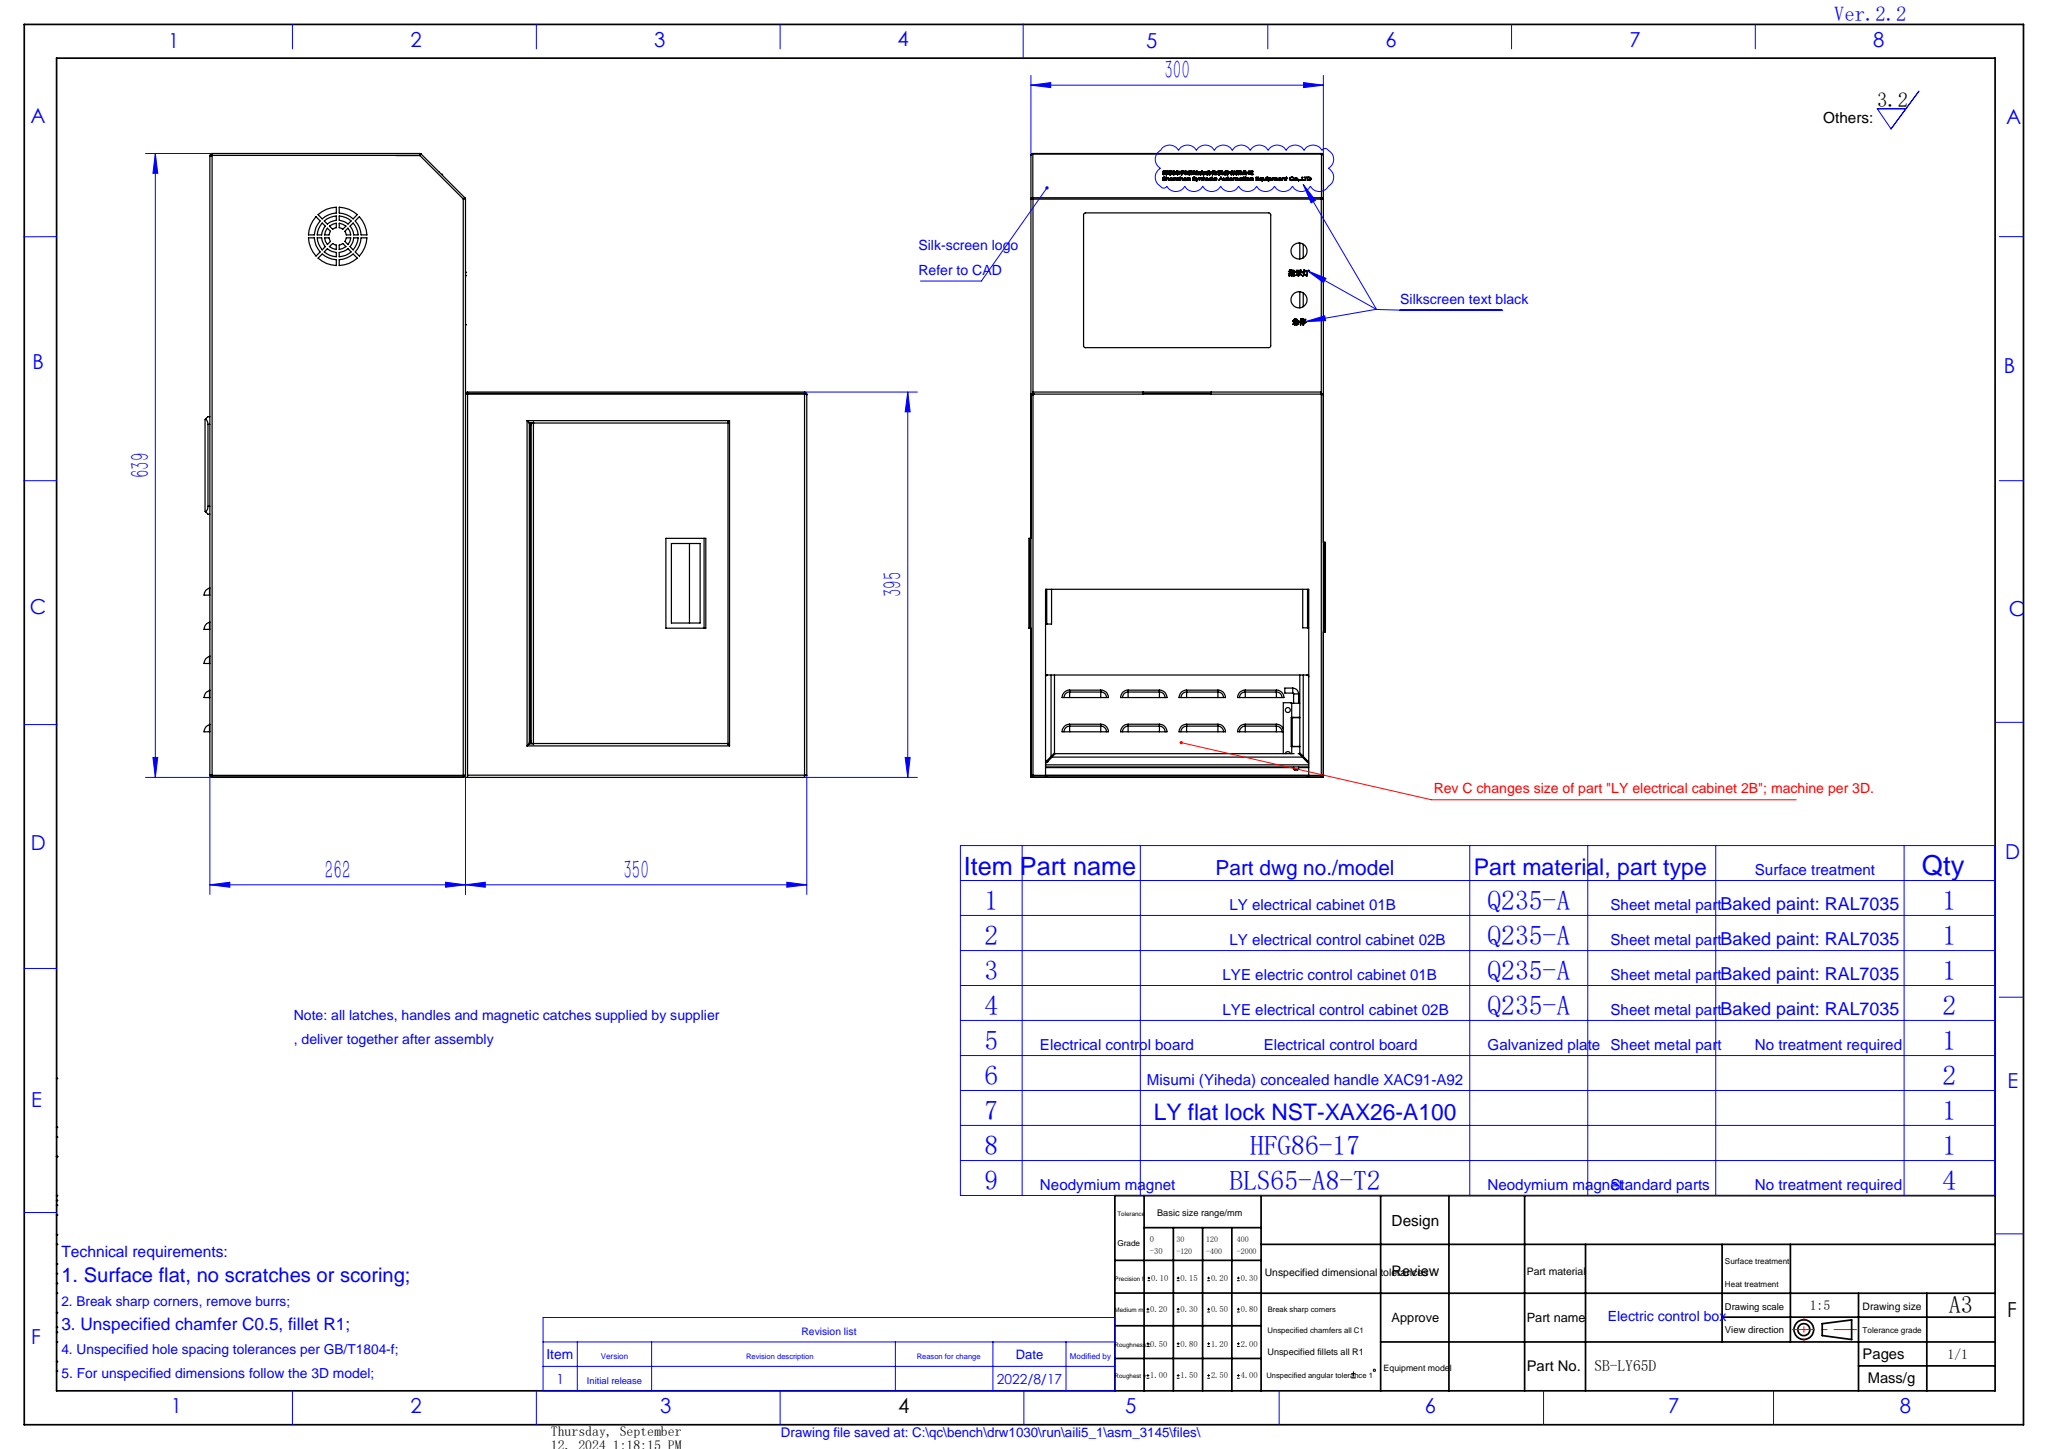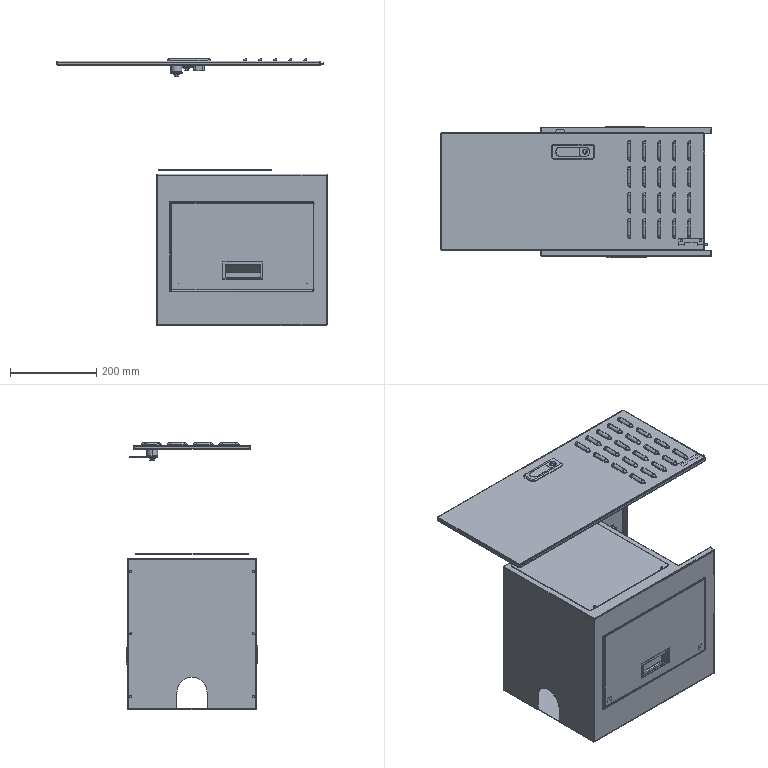Part | SolidWorks | features CompositeCurve 2, LocalLPattern 2, ReferencePattern 2 | 14 solids | 1198 faces | box 625.233 x 304 x 617.993 mm | volume 1412506 mm3 | plane 569 | cylinder 331 | spline 94 | torus 82 | sphere 80 | cone 42 | commonest cylinder face diameters 1.473 x49 4.473 x49 4 x36 5 x30 1 x20 12 x20